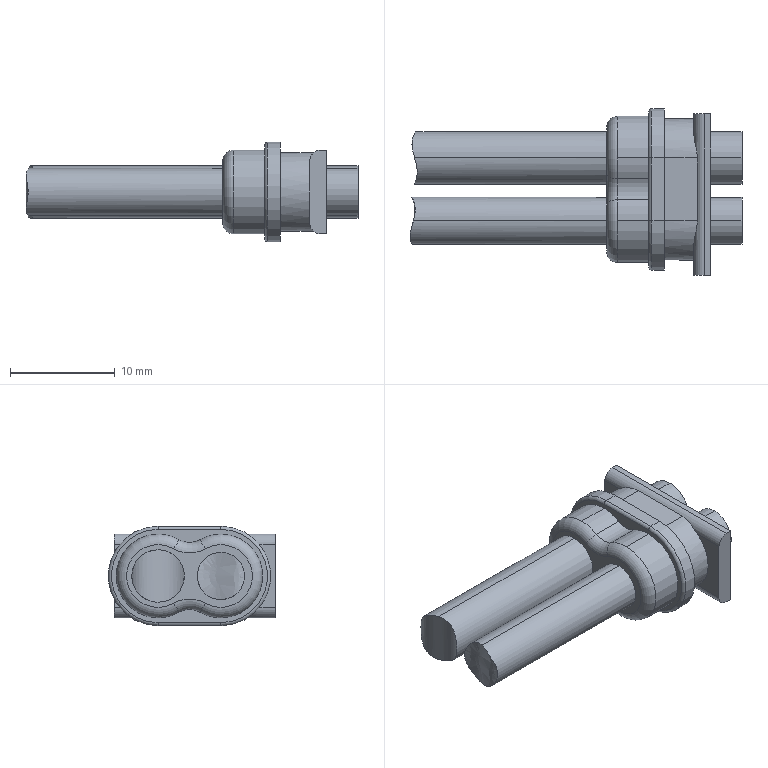Part | SolidWorks | features BaseBody 1 | 1 solid | 49 faces | box 31.691 x 15.95 x 9.5 mm | volume 1762 mm3 | cylinder 25 | plane 16 | torus 6 | spline 2 | commonest cylinder face diameters 8 x6 4.5 x4 5 x4 4 x3 0.6 x2 2 x2